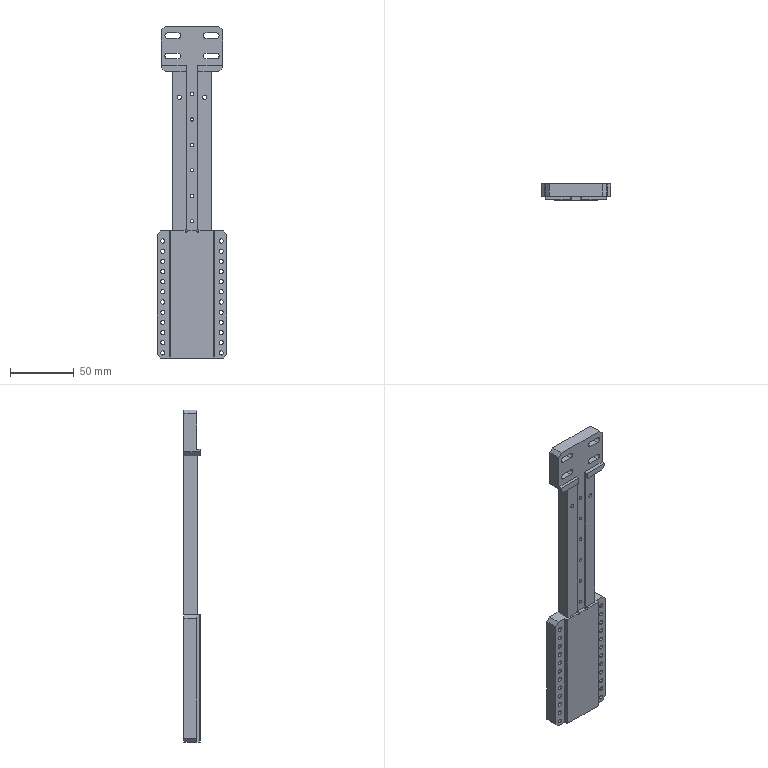Part | SolidWorks | features ICE 9, HoleWzd 4, Chamfer 3, LPattern 2, 3DProfileFeature 1, Extrusion 1, MirrorPattern 1 | 1 solid | 126 faces | box 55 x 12.8 x 261 mm | volume 117681 mm3 | cylinder 78 | plane 46 | cone 2 | commonest cylinder face diameters 3.3 x52 2.5 x14 4.5 x8 2 x4